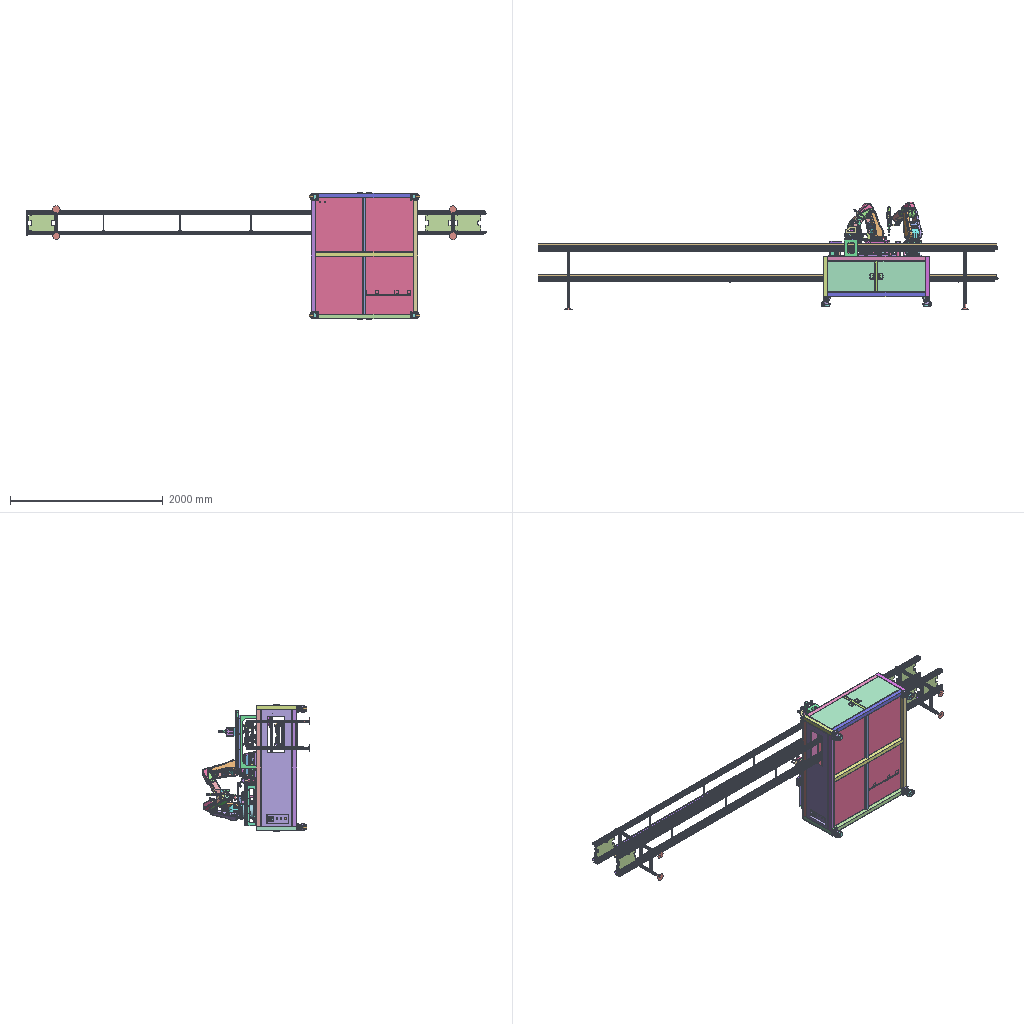Assembly | STEP file | 266 different items | 520 placed | box 6033 x 1412 x 1658 mm
Parts list (item | name | quantity | parent item | size | volume):
1 | ASND-0110-IRB120_3-58_IRC5_Link2_rev0 | x2 | in ASND-0110-B, ASND-0110-B-1 | 144.86 x 219.43 x 390.86 mm | 3910323 mm3
2 | ASND-0110-IRB120_3-58_IRC5_Link5_rev0 | x2 | in ASND-0110-C, ASND-0110-C-1 | 51 x 61.424 x 80.382 mm | 189880 mm3
3 | ASND-0110-IRB120_3-58_IRC5_Link5_rev0-1 | x2 | in ASND-0110-C, ASND-0110-C-1 | 21.5 x 70 x 70 mm | 66105 mm3
4 | ASND-0110-IRB120_3-58_IRC5_Link5_rev0-2 | x2 | in ASND-0110-C, ASND-0110-C-1 | 62.5 x 72 x 82 mm | 291195 mm3
5 | ASND-0110-IRB120_3-58_IRC5_Link4_rev0 | x2 | in ASND-0110-A, ASND-0110-A-1 | 193.368 x 85.5 x 92.955 mm | 549837 mm3
6 | ASND-0110-IRB120_3-58_IRC5_Link3_rev0 | x2 | in ASND-0110-A, ASND-0110-A-1 | 10 x 96 x 96 mm | 36166 mm3
7 | ASND-0110-IRB120_3-58_IRC5_Link4_rev0-1 | x2 | in ASND-0110-A, ASND-0110-A-1 | 111.545 x 11.377 x 37.543 mm | 181.054 mm3
8 | ASND-0110-IRB120_3-58_IRC5_Link4_rev0-2 | x2 | in ASND-0110-A, ASND-0110-A-1 | 186.08 x 124 x 105.45 mm | 774376 mm3
9 | ASND-0110-IRB120_3-58_IRC5_Link3_rev0-1 | x2 | in ASND-0110-E, ASND-0110-E-1 | 233.871 x 115.5 x 188.155 mm | 2907846 mm3
10 | ASND-0110-IRB120_3-58_IRC5_Base_rev0 | x2 | in ASND-0110-First axis, ASND-0110-First axisB | 301.2 x 180.524 x 166.334 mm | 6215073 mm3
11 | ASND-0110-IRB120_3-58_IRC5_Link1_rev0-1 | x2 | in ASND-0110-First axis, ASND-0110-First axisB | 215 x 215 x 22 mm | 381566 mm3
12 | ASND-0110-Body 1-1 | x1 | in ASND-0110-D1 | 280 x 240 x 15 mm | 976987 mm3
13 | ASND-0110-Body 1-2 | x1 | in ASND-0110-D | 280 x 220 x 15 mm | 890688 mm3
14 | ASND-0110-Body 1-5 | x4 | in ASND-0110-asd | 5 x 5 x 2.3 mm | 45.16 mm3
15 | ASND-0110-TPIM-023 | x1 | in ASND-0110-asd | 111.9 x 71.3 x 30 mm | 98030 mm3
16 | ASND-0110-IRB120_Link6_rev0 | x2 | in ASND-0110-Robot suction mechanism, ASND-0110-Screw locking mechanism | 13 x 40 x 40 mm | 13678 mm3
17 | ASND-0110-Body 1-3 | x8 | in ASND-0110-Robot suction mechanism, ASND-0110-XXY mechanism | 20 x 20 x 10 mm | 1461 mm3
18 | ASND-0110-TPIM-022 | x1 | in ASND-0110-Robot suction mechanism | 248.345 x 15 x 75.4 mm | 86870 mm3
19 | ASND-0110-TPIM-020 | x1 | in ASND-0110-Robot suction mechanism | 92 x 92 x 18 mm | 89646 mm3
20 | ASND-0110-YD02 | x2 | in ASND-0110-Robot suction mechanism | 66 x 64 x 12.7 mm | 33292 mm3
21 | ASND-0110-TPIM-068 | x1 | in ASND-0110-Robot suction mechanism | 46.8 x 34.8 x 15.8 mm | 14684 mm3
22 | ASND-0110-Solid1 | x1 | in ASND-0110-Robot suction mechanism | 20.8 x 7 x 7 mm | 257.271 mm3
23 | ASND-0110-TPIM-标定01 | x1 | in ASND-0110-Robot suction mechanism | 24 x 14 x 6 mm | 2012 mm3
24 | ASND-0110-Body 1-4 | x1 | in ASND-0110-Robot suction mechanism | 83 x 53 x 7 mm | 13678 mm3
25 | ASND-0110-HI_Motor--01-APAAa5wgTCTF01 | x1 | in ASND-0110-MAMS012G1ATCTF01 | 117.03 x 38.2 x 38.2 mm | 124253 mm3
26 | ASND-0110-HI_Motoplug--01ATCTF01 | x1 | in ASND-0110-MAMS012G1ATCTF01 | 27 x 33.5 x 37.535 mm | 8192 mm3
27 | ASND-0110-HI_Cabel Motoplug--01PTCTF01 | x1 | in ASND-0110-MAMS012G1ATCTF01 | 9 x 52.5 x 9 mm | 1909 mm3
28 | ASND-0110-HI_Motor ConnectorTCTF01 | x1 | in ASND-0110-MAMS012G1ATCTF01 | 23.7 x 14.7 x 9.8 mm | 1306 mm3
29 | ASND-0110-HI_Encoder--01PTCTF01 | x1 | in ASND-0110-MAMS012G1ATCTF01 | 30.365 x 32.633 x 22.9 mm | 5926 mm3
30 | ASND-0110-HI_Cabel  brake--01-P-4TCTF01 | x1 | in ASND-0110-MAMS012G1ATCTF01 | 7.2 x 36.535 x 7.2 mm | 1162 mm3
31 | ASND-0110-HI_2500 p_r ConnectorTCTF01 | x1 | in ASND-0110-MAMS012G1ATCTF01 | 23.7 x 14.7 x 14.5 mm | 2117 mm3
32 | ASND-0110-KK60-500 | x1 | in ASND-0110-KK60-500A1-F0 | 570 x 44.5 x 60 mm | 511648 mm3
33 | ASND-0110-KK60-A1 | x1 | in ASND-0110-KK60-500A1-F0 | 82 x 21 x 51.857 mm | 53460 mm3
34 | ASND-0110-TCTF01-28 | x1 | in ASND-0110-KK module TCTF01(default-_flexible1) | 12 x 50 x 44 mm | 18847 mm3
35 | ASND-0110-KK6010P-600A1-F1CS1-8TCTF01 | x1 | in ASND-0110-KK module TCTF01(default-_flexible1) | 500 x 8 x 5 mm | 9828 mm3
36 | ASND-0110-HGR15_1TCTF01sb | x1 | in ASND-0110-HGR15_1TCTF01 | 15 x 15 x 530 mm | 97544 mm3
37 | ASND-0110-TCTF01-31 | x1 | in ASND-0110-Tooling mechanism | 90 x 51 x 22 mm | 59920 mm3
38 | ASND-0110-Body 1-9 | x1 | in ASND-0110-Tooling mechanism | 160 x 114 x 12 mm | 207606 mm3
39 | ASND-0110-Body 1-10 | x1 | in ASND-0110-Tooling mechanism | 160 x 114 x 25 mm | 365953 mm3
40 | ASND-0110-DH2TC90-28(2) | x1 | in ASND-0110-Tooling mechanism | 15 x 30 x 16.25 mm | 397.632 mm3
41 | ASND-0110-HGH15_2TCTF01sb | x1 | in ASND-0110-Tooling mechanism | 34 x 23.7 x 61.4 mm | 36561 mm3
42 | ASND-0110-KK60-A1gf4 | x1 | in ASND-0110-Tooling mechanism | 82 x 21 x 51.857 mm | 53460 mm3
43 | - | x1 | in ASND-0110-Tooling mechanism | 13 x 52 x 15.011 mm | 2605 mm3
44 | ASND-0110-Body 1-11 | x1 | in ASND-0110-Tooling mechanism | 80 x 22 x 35 mm | 6854 mm3
45 | ASND-0110-TCTF01-29 | x1 | in ASND-0110-Feeding mechanism | 70 x 101.1 x 530 mm | 1817903 mm3
46 | ASND-0110-TCTF01-34 | x1 | in ASND-0110-Feeding mechanism | 530 x 32 x 127.1 mm | 1195079 mm3
47 | ASND-0110-TCTF01-30(default) | x1 | in ASND-0110-Feeding mechanism | 522 x 1.5 x 56 mm | 43747 mm3
48 | ASND-0110-Body 1-6 | x1 | in ASND-0110-Feeding mechanism | 550 x 32 x 10 mm | 26590 mm3
49 | ASND-0110-Positioning edgeHSG side gTCTF01 | x2 | in ASND-0110-Feeding mechanism | 6 x 6 x 14 mm | 362.314 mm3
50 | ASND-0110-Body 1-7 | x1 | in ASND-0110-Feeding mechanism | 22 x 79.611 x 439.805 mm | 70298 mm3
51 | ASND-0110-Body 1-8 | x1 | in ASND-0110-Feeding mechanism | 202 x 550 x 12 mm | 1322271 mm3
52 | ASND-0110-1 | x2 | in ASND-0110-Rotary clamping mechanism, ASND-0110-Revolve夹持机构-1 | 29 x 29 x 68 mm | 33970 mm3
53 | ASND-0110-clamp 12 | x2 | in ASND-0110-Rotary clamping mechanism, ASND-0110-Revolve夹持机构-1 | 87 x 17 x 20 mm | 14618 mm3
54 | ASND-0110-Body 1-14 | x2 | in ASND-0110-Rotary clamping mechanism, ASND-0110-Revolve夹持机构-1 | 20 x 12 x 2 mm | 472 mm3
55 | ASND-0110-Surface 1-1 | x1 | in ASND-0110-XXY mechanism | - | -
56 | ASND-0110-TCTF01-24 | x1 | in ASND-0110-XXY mechanism | 366.812 x 377.833 x 20 mm | 1326662 mm3
57 | ASND-0110-TCTF01-23 | x1 | in ASND-0110-XXY mechanism | 366.812 x 377.833 x 16 mm | 1379157 mm3
58 | ASND-0110-TCTF01-35 | x1 | in ASND-0110-XXY mechanism | 317.501 x 248.833 x 21 mm | 1208594 mm3
59 | ASND-0110-TCTF01-58 | x1 | in ASND-0110-XXY mechanism | 256.83 x 10 x 30 mm | 53115 mm3
60 | ASND-0110-TCTF01-57 | x1 | in ASND-0110-XXY mechanism | 78 x 30 x 10 mm | 20925 mm3
61 | ASND-0110-TCTF01-57-1 | x1 | in ASND-0110-XXY mechanism | 92 x 30 x 10 mm | 25160 mm3
62 | ASND-0110-Body 1-12 | x2 | in ASND-0110-XXY mechanism | 66 x 29 x 8 mm | 12885 mm3
63 | ASND-0110-Body 1-13 | x1 | in ASND-0110-XXY mechanism | 366.812 x 370.85 x 30 mm | 2210329 mm3
64 | ASND-0110-Solid1-1 | x1 | in ASND-0110-XXY mechanism | 12.3 x 7 x 7 mm | 177.16 mm3
65 | ASND-0110-PG Flea2 | x6 | in ASND-0110-Camera mechanisma, ASND-0110-Camera mechanisma-1, ASND-0110-Camera mechanisma-2, ASND-0110-Camera mechanisma-3, ASND-0110-Camera section, ASND-0110-相机部分-1 | 29 x 29 x 47.1 mm | 26811 mm3
66 | ASND-0110-Body 1-15 | x4 | in ASND-0110-Camera mechanisma, ASND-0110-Camera mechanisma-1, ASND-0110-Camera mechanisma-2, ASND-0110-Camera mechanisma-3 | 40.5 x 29 x 94 mm | 35874 mm3
67 | ASND-0110-Surface 1-2 | x1 | in ASND-0110-tiaoj | - | -
68 | ASND-0110-OPT-CO40-X-V1.0.5 mounting plate | x4 | in ASND-0110-OPT-CO40-X-V1.0.5, ASND-0110-OPT-CO40-X-V1.0.5_1, ASND-0110-OPT-CO40-X-V1.0.5_2, ASND-0110-OPT-CO40-X-V1.0.5_3 | 32 x 39 x 8 mm | 9600 mm3
69 | ASND-0110-OPT-CO40-X-V1.0.5 side plate | x4 | in ASND-0110-OPT-CO40-X-V1.0.5, ASND-0110-OPT-CO40-X-V1.0.5_1, ASND-0110-OPT-CO40-X-V1.0.5_2, ASND-0110-OPT-CO40-X-V1.0.5_3 | 69 x 39 x 4 mm | 10181 mm3
70 | ASND-0110-OPT-CO40-X-V1.0 rear cover plate | x4 | in ASND-0110-OPT-CO40-X-V1.0.5, ASND-0110-OPT-CO40-X-V1.0.5_1, ASND-0110-OPT-CO40-X-V1.0.5_2, ASND-0110-OPT-CO40-X-V1.0.5_3 | 32 x 35 x 5 mm | 5286 mm3
71 | ASND-0110-OPT-CO40-X-V1.0 upper cover plate | x4 | in ASND-0110-OPT-CO40-X-V1.0.5, ASND-0110-OPT-CO40-X-V1.0.5_1, ASND-0110-OPT-CO40-X-V1.0.5_2, ASND-0110-OPT-CO40-X-V1.0.5_3 | 34 x 29 x 2 mm | 1761 mm3
72 | ASND-0110-OPT-CO40-X-V1.0 lower cover plate | x4 | in ASND-0110-OPT-CO40-X-V1.0.5, ASND-0110-OPT-CO40-X-V1.0.5_1, ASND-0110-OPT-CO40-X-V1.0.5_2, ASND-0110-OPT-CO40-X-V1.0.5_3 | 34 x 25.2 x 2 mm | 1591 mm3
73 | ASND-0110-OPT-CO40-X-V1.0 diffuser plate | x4 | in ASND-0110-OPT-CO40-X-V1.0.5, ASND-0110-OPT-CO40-X-V1.0.5_1, ASND-0110-OPT-CO40-X-V1.0.5_2, ASND-0110-OPT-CO40-X-V1.0.5_3 | 34.8 x 34.2 x 2 mm | 2380 mm3
74 | ASND-0110-Mirrored OPT-CO40-X-V1.0 side plate | x4 | in ASND-0110-OPT-CO40-X-V1.0.5, ASND-0110-OPT-CO40-X-V1.0.5_1, ASND-0110-OPT-CO40-X-V1.0.5_2, ASND-0110-OPT-CO40-X-V1.0.5_3 | 69 x 39 x 4 mm | 10181 mm3
75 | ASND-0110-2-core power cable | x4 | in ASND-0110-OPT-CO40-X-V1.0.5, ASND-0110-OPT-CO40-X-V1.0.5_1, ASND-0110-OPT-CO40-X-V1.0.5_2, ASND-0110-OPT-CO40-X-V1.0.5_3 | 15 x 5 x 19.875 mm | 201.3 mm3
76 | ASND-0110-TPIM-067 | x2 | in ASND-0110-Lower light source mechanism | 55.8 x 8 x 39 mm | 15980 mm3
77 | ASND-0110-TPIM-065 | x1 | in ASND-0110-Lower light source mechanism | 160 x 111.5 x 30 mm | 146139 mm3
78 | ASND-0110-TPIM-066 | x1 | in ASND-0110-Lower light source mechanism | 132.4 x 10 x 159 mm | 81070 mm3
79 | ASND-0110-Body 1-16 | x2 | in ASND-0110-Lower camera mechanism | 120 x 120 x 10 mm | 61912 mm3
80 | ASND-0110-Body 1-17 | x1 | in ASND-0110-Lower camera mechanism | 128 x 216 x 10 mm | 155040 mm3
81 | ASND-0110-Body 1-18 | x2 | in ASND-0110-Lower camera mechanism | 30 x 31 x 10 mm | 8202 mm3
82 | ASND-0110-Body 1-19 | x2 | in ASND-0110-Lower camera mechanism | 30 x 31 x 10 mm | 8202 mm3
83 | ASND-0110-Body 1-20 | x1 | in ASND-0110-Lower camera mechanism | 178 x 128 x 72 mm | 360301 mm3
84 | ASND-0110-Body 1-21 | x2 | in ASND-0110-Lower camera mechanism | 80 x 52 x 18 mm | 53842 mm3
85 | ASND-0110-4216100000 | x1 | in ASND-0110-4216100080_ASM | 30 x 30 x 163.75 mm | 53858 mm3
86 | ASND-0110-4216107200 | x1 | in ASND-0110-4216100080_ASM | 25 x 18 x 16 mm | 3261 mm3
87 | ASND-0110-Surface 1-3 | x1 | in ASND-0110-4216100080_ASM | - | -
88 | ASND-0110-4216107480_SPEC | x1 | in ASND-0110-4216100080_ASM | 15.011 x 14 x 14 mm | 1337 mm3
89 | ASND-0110-Surface 1-4 | x1 | in ASND-0110-4216100080_ASM | - | -
90 | ASND-0110-0219110005 | x2 | in ASND-0110-4216100080_ASM | 4.7 x 4.7 x 20 mm | 105.896 mm3
91 | ASND-0110-Surface 1-5 | x2 | in ASND-0110-4216100080_ASM | - | -
92 | ASND-0110-4216101100 | x1 | in ASND-0110-4224300000_ASM | 25 x 116.5 x 18 mm | 12649 mm3
93 | ASND-0110-4216225600 | x1 | in ASND-0110-4224300000_ASM | 29 x 29 x 58 mm | 3832 mm3
94 | ASND-0110-0162110302 | x2 | in ASND-0110-4224300000_ASM | 3 x 3 x 12 mm | 26.529 mm3
95 | ASND-0110-Surface 1-6 | x2 | in ASND-0110-4224300000_ASM | - | -
96 | ASND-0110-0219110003 | x2 | in ASND-0110-4224300000_ASM | 5.5 x 5.5 x 12 mm | 96.355 mm3
97 | ASND-0110-Surface 1-7 | x2 | in ASND-0110-4224300000_ASM | - | -
98 | ASND-0110-0219110001 | x2 | in ASND-0110-4224300000_ASM | 5 x 4.7 x 4.7 mm | 32.246 mm3
99 | ASND-0110-0219110027 | x1 | in ASND-0110-4224300000_ASM | 6 x 6 x 6 mm | 55.363 mm3
100 | ASND-0110-Surface 1-8 | x1 | in ASND-0110-4224300000_ASM | - | -
101 | ASND-0110-4216235500_SPEC | x1 | in ASND-0110-4224300000_ASM | 29.395 x 14.422 x 30 mm | 229.451 mm3
102 | ASND-0110-4216111600 | x1 | in ASND-0110-4224300001_ASM | 9 x 9 x 56.7 mm | 1924 mm3
103 | ASND-0110-4216111500 | x1 | in ASND-0110-4224300001_ASM | 10 x 10 x 6 mm | 119.565 mm3
104 | ASND-0110-4216111700 | x1 | in ASND-0110-4224300001_ASM | 9 x 9 x 9 mm | 120.166 mm3
105 | ASND-0110-0502110051 | x1 | in ASND-0110-4224300001_ASM | 4 x 15.6 x 15.6 mm | 444.035 mm3
106 | ASND-0110-4216109900 | x1 | in ASND-0110-4224300001_ASM | 25 x 25 x 33.65 mm | 5833 mm3
107 | ASND-0110-Surface 1-9 | x1 | in ASND-0110-4224300001_ASM | - | -
108 | ASND-0110-4216111200_SPEC_AF0 | x1 | in ASND-0110-4224300001_ASM | 8.7 x 8.7 x 5.55 mm | 29.663 mm3
109 | ASND-0110-4216111400_AF0 | x1 | in ASND-0110-4224300001_ASM | 8.635 x 8.7 x 1 mm | 17.813 mm3
110 | ASND-0110-Screw gunpart1 | x1 | in ASND-0110-螺丝枪1 | 6.827 x 116 x 6.827 mm | 2290 mm3
111 | ASND-0110-Surface 1-10 | x1 | in ASND-0110-atlas-A | - | -
112 | ASND-0110-Surface 1_1 | x1 | in ASND-0110-atlas-A | - | -
113 | ASND-0110-Surface 1_2 | x1 | in ASND-0110-atlas-A | - | -
114 | ASND-0110-Body 1-22 | x1 | in ASND-0110-Screw locking mechanism | 48 x 48 x 13 mm | 15905 mm3
115 | ASND-0110-Body 1-23 | x1 | in ASND-0110-Screw locking mechanism | 65 x 40 x 6 mm | 15450 mm3
116 | ASND-0110-BAIF-08 | x1 | in ASND-0110-Screw locking mechanism | 104 x 84 x 15 mm | 94605 mm3
117 | ASND-0110-Body 1-1-1 | x1 | in ASND-0110-Screw locking mechanism | 120 x 34 x 8 mm | 32440 mm3
118 | ASND-0110-PG Flea2-1 | x1 | in ASND-0110-Screw locking mechanism | 32 x 32 x 92.1 mm | 40913 mm3
119 | ASND-0110-Body 1-1ww | x1 | in ASND-0110-Screw locking mechanism | 84 x 119.7 x 12 mm | 119908 mm3
120 | ASND-0110-SDS_3 | x1 | in ASND-0110-SDS_SR | 181.1 x 144.1 x 117 mm | 1395902 mm3
121 | ASND-0110-SDS_3_1 | x1 | in ASND-0110-SDS_SR | 1 x 24.6 x 24 mm | 538.331 mm3
122 | ASND-0110-SDS_1 | x1 | in ASND-0110-SDS_SR | 181 x 139 x 3 mm | 64643 mm3
123 | ASND-0110-SDS_2 | x1 | in ASND-0110-SDS_SR | 181 x 139 x 3 mm | 64643 mm3
124 | ASND-0110-SDS_4 | x1 | in ASND-0110-SDS_SR | 122.6 x 80.2 x 5 mm | 16643 mm3
125 | ASND-0110-0162156729 | x16 | in ASND-0110-SDS_SR | 7.5 x 7.5 x 10 mm | 160.064 mm3
126 | ASND-0110-SDS_5 | x1 | in ASND-0110-SDS_SR | 2 x 38.8 x 73.5 mm | 3386 mm3
127 | ASND-0110-SDS_6 | x1 | in ASND-0110-SDS_SR | 31.924 x 31.924 x 2 mm | 1536 mm3
128 | ASND-0110-SDS_7 | x1 | in ASND-0110-SDS_SR | 57.4 x 48.5 x 8.5 mm | 3034 mm3
129 | ASND-0110-SDS_8 | x1 | in ASND-0110-SDS_SR | 22 x 30.4 x 12 mm | 1042 mm3
130 | ASND-0110-SDS_9 | x1 | in ASND-0110-SDS_SR | 21.7 x 12.9 x 40 mm | 1125 mm3
131 | ASND-0110-0211110400 | x2 | in ASND-0110-SDS_SR | 9 x 5.5 x 5.5 mm | 106.119 mm3
132 | ASND-0110-0211110210 | x2 | in ASND-0110-SDS_SR | 6 x 3.8 x 3.8 mm | 33.139 mm3
133 | ASND-0110-0211110266 | x2 | in ASND-0110-SDS_SR | 4.5 x 4.5 x 8.5 mm | 65.135 mm3
134 | ASND-0110-Surface 1-11 | x2 | in ASND-0110-SDS_SR | - | -
135 | ASND-0110-0160099710 | x2 | in ASND-0110-SDS_SR | 3.2 x 3.2 x 4.4 mm | 13.426 mm3
136 | ASND-0110-Surface 1-12 | x2 | in ASND-0110-SDS_SR | - | -
137 | ASND-0110-Body 1-24 | x1 | in ASND-0110-Screw feeding mechanism | 181 x 123 x 100 mm | 983865 mm3
138 | ASND-0110-OPT-CO60-X-V1.0 front cover plate | x2 | in ASND-0110-OPT-CO60-X-V1.0, ASND-0110-OPT-CO60-X-V1.0-1 | 50 x 57.4 x 8 mm | 21783 mm3
139 | ASND-0110-OPT-CO60-X-V1.0 side plate | x2 | in ASND-0110-OPT-CO60-X-V1.0, ASND-0110-OPT-CO60-X-V1.0-1 | 90 x 57.4 x 4 mm | 19730 mm3
140 | ASND-0110-OPT-CO60-X-V1.0 rear cover plate | x2 | in ASND-0110-OPT-CO60-X-V1.0, ASND-0110-OPT-CO60-X-V1.0-1 | 50 x 53 x 5 mm | 13081 mm3
141 | ASND-0110-OPT-CO60-X-V1.0 upper cover plate | x2 | in ASND-0110-OPT-CO60-X-V1.0, ASND-0110-OPT-CO60-X-V1.0-1 | 31 x 52.3 x 2.2 mm | 3229 mm3
142 | ASND-0110-OPT-CO60-X-V1.0 lower cover plate | x2 | in ASND-0110-OPT-CO60-X-V1.0, ASND-0110-OPT-CO60-X-V1.0-1 | 2.2 x 27 x 52.3 mm | 2996 mm3
143 | ASND-0110-2-core outlet terminal | x2 | in ASND-0110-OPT-CO60-X-V1.0, ASND-0110-OPT-CO60-X-V1.0-1 | 27 x 10 x 28.25 mm | 1155 mm3
144 | ASND-0110-Mirrored OPT-CO60-X-V1.0 side plate | x2 | in ASND-0110-OPT-CO60-X-V1.0, ASND-0110-OPT-CO60-X-V1.0-1 | 90 x 57.4 x 4 mm | 19730 mm3
145 | ASND-0110-Body 1-25 | x2 | in ASND-0110-Camera section, ASND-0110-相机部分-1 | 75 x 87.1 x 55 mm | 96917 mm3
146 | ASND-0110-相机连接件2 | x2 | in ASND-0110-Camera section, ASND-0110-相机部分-1 | 75 x 139 x 10 mm | 83120 mm3
147 | ASND-0110-Camera base block | x2 | in ASND-0110-Camera section, ASND-0110-相机部分-1 | 54 x 50 x 14 mm | 21543 mm3
148 | ASND-0110-TPIM-064 | x2 | in ASND-0110-Camera section, ASND-0110-相机部分-1 | 11.6 x 176 x 58 mm | 99143 mm3
149 | ASND-0110-Lens | x2 | in ASND-0110-Camera section, ASND-0110-相机部分-1 | 46 x 141.1 x 46 mm | 154074 mm3
150 | ASND-0110-1-1 | x2 | in ASND-0110-2-25, ASND-0110-2-25-1 | 30 x 30 x 749.1 mm | 248521 mm3
151 | ASND-0110-1-2 | x2 | in ASND-0110-2-25, ASND-0110-2-25-1 | 30 x 30 x 749.1 mm | 248521 mm3
152 | ASND-0110-1-3 | x2 | in ASND-0110-2-25, ASND-0110-2-25-1 | 30 x 320 x 30 mm | 106163 mm3
153 | ASND-0110-1-4 | x4 | in ASND-0110-2-25, ASND-0110-2-25-1 | 30 x 320 x 30 mm | 106163 mm3
154 | ASND-0110-1.120ww | x4 | in ASND-0110-2-25, ASND-0110-2-25-1 | 96.056 x 88 x 96.056 mm | 106190 mm3
155 | ASND-0110-PWP TOP tu pang 20130814.sldasm-Part-1aq (subassembly) | x7 | in ASND-0110-Tray aq, ASND-0110-Tray aq-1, ASND-0110-Tray aq-2, ASND-0110-Tray aq-3, ASND-0110-Tray aq-4, ASND-0110-Tray aq-5, ASND-0110-Tray aq-6 | 256 x 10 x 12 mm | 28147 mm3
156 | ASND-0110-PWP TOP tu pang 20130814.sldasm-Part-2aq (subassembly) | x7 | in ASND-0110-Tray aq, ASND-0110-Tray aq-1, ASND-0110-Tray aq-2, ASND-0110-Tray aq-3, ASND-0110-Tray aq-4, ASND-0110-Tray aq-5, ASND-0110-Tray aq-6 | 337.093 x 249.456 x 14.1 mm | 1124942 mm3
157 | ASND-0110-PWP TOP tu pang 20130814.sldasm-Part-5aq (subassembly) | x7 | in ASND-0110-Tray aq, ASND-0110-Tray aq-1, ASND-0110-Tray aq-2, ASND-0110-Tray aq-3, ASND-0110-Tray aq-4, ASND-0110-Tray aq-5, ASND-0110-Tray aq-6 | 40.426 x 89.575 x 12 mm | 15056 mm3
158 | ASND-0110-PWP TOP tu pang 20130814.sldasm-Part-6aq (subassembly) | x7 | in ASND-0110-Tray aq, ASND-0110-Tray aq-1, ASND-0110-Tray aq-2, ASND-0110-Tray aq-3, ASND-0110-Tray aq-4, ASND-0110-Tray aq-5, ASND-0110-Tray aq-6 | 40.426 x 89.575 x 12 mm | 15056 mm3
159 | ASND-0110-PWP TOP tu pang 20130814.sldasm-Part-7aq (subassembly) | x7 | in ASND-0110-Tray aq, ASND-0110-Tray aq-1, ASND-0110-Tray aq-2, ASND-0110-Tray aq-3, ASND-0110-Tray aq-4, ASND-0110-Tray aq-5, ASND-0110-Tray aq-6 | 31.546 x 101 x 12 mm | 15497 mm3
160 | ASND-0110-PWP TOP tu pang 20130814.sldasm-Part-8aq (subassembly) | x7 | in ASND-0110-Tray aq, ASND-0110-Tray aq-1, ASND-0110-Tray aq-2, ASND-0110-Tray aq-3, ASND-0110-Tray aq-4, ASND-0110-Tray aq-5, ASND-0110-Tray aq-6 | 305.546 x 101 x 12 mm | 72445 mm3
161 | ASND-0110-Q1 | x2 | in ASND-0110-Upper streamline, ASND-0110-Upper流线-1 | 5993 x 32 x 186 mm | 1783036 mm3
162 | ASND-0110-Q2 | x2 | in ASND-0110-Upper streamline, ASND-0110-Upper流线-1 | 6033 x 32.8 x 10 mm | 266115 mm3
163 | ASND-0110-Q3 | x2 | in ASND-0110-Upper streamline, ASND-0110-Upper流线-1 | 6033 x 32.8 x 10 mm | 266115 mm3
164 | ASND-0110-Q20 | x2 | in ASND-0110-Upper streamline, ASND-0110-Upper流线-1 | 11.547 x 10 x 18 mm | 731.296 mm3
165 | ASND-0110-Q20_1 | x2 | in ASND-0110-Upper streamline, ASND-0110-Upper流线-1 | 38 x 16 x 227.5 mm | 31386 mm3
166 | ASND-0110-Q20_2 | x2 | in ASND-0110-Upper streamline, ASND-0110-Upper流线-1 | 11.547 x 10 x 18 mm | 731.296 mm3
167 | ASND-0110-Q21 | x2 | in ASND-0110-Upper streamline, ASND-0110-Upper流线-1 | 11.547 x 10 x 18 mm | 731.296 mm3
168 | ASND-0110-Q21_1 | x2 | in ASND-0110-Upper streamline, ASND-0110-Upper流线-1 | 38 x 16 x 227.5 mm | 31386 mm3
169 | ASND-0110-Q21_2 | x2 | in ASND-0110-Upper streamline, ASND-0110-Upper流线-1 | 11.547 x 10 x 18 mm | 731.296 mm3
170 | ASND-0110-Q22 | x6 | in ASND-0110-Upper streamline, ASND-0110-Upper流线-1 | 11.547 x 10 x 18 mm | 731.296 mm3
171 | ASND-0110-Q22_1 | x6 | in ASND-0110-Upper streamline, ASND-0110-Upper流线-1 | 38 x 16 x 227.5 mm | 31386 mm3
172 | ASND-0110-Q22_2 | x6 | in ASND-0110-Upper streamline, ASND-0110-Upper流线-1 | 11.547 x 10 x 18 mm | 731.296 mm3
173 | ASND-0110-Q23 | x2 | in ASND-0110-Upper streamline, ASND-0110-Upper流线-1 | 40 x 52 x 28.5 mm | 23081 mm3
174 | ASND-0110-Q26 | x2 | in ASND-0110-Upper streamline, ASND-0110-Upper流线-1 | 40 x 52 x 28.5 mm | 23081 mm3
175 | ASND-0110-Q27 | x2 | in ASND-0110-Upper streamline, ASND-0110-Upper流线-1 | 40 x 52 x 28.5 mm | 23081 mm3
176 | ASND-0110-Q29 | x2 | in ASND-0110-Upper streamline, ASND-0110-Upper流线-1 | 6.351 x 5.5 x 2.4 mm | 50.688 mm3
177 | ASND-0110-Q30 | x2 | in ASND-0110-Upper streamline, ASND-0110-Upper流线-1 | 11.5 x 10 x 5 mm | 332.096 mm3
178 | ASND-0110-Q31 | x2 | in ASND-0110-Upper streamline, ASND-0110-Upper流线-1 | 11.5 x 10 x 5 mm | 332.096 mm3
179 | ASND-0110-Q32 | x2 | in ASND-0110-Upper streamline, ASND-0110-Upper流线-1 | 6.351 x 5.5 x 2.4 mm | 50.688 mm3
180 | ASND-0110-Q33 | x2 | in ASND-0110-Upper streamline, ASND-0110-Upper流线-1 | 6.351 x 5.5 x 2.4 mm | 50.688 mm3
181 | ASND-0110-Q34 | x2 | in ASND-0110-Upper streamline, ASND-0110-Upper流线-1 | 11.5 x 10 x 5 mm | 332.096 mm3
182 | ASND-0110-Q35 | x2 | in ASND-0110-Upper streamline, ASND-0110-Upper流线-1 | 11.5 x 10 x 5 mm | 332.096 mm3
183 | ASND-0110-Q36 | x2 | in ASND-0110-Upper streamline, ASND-0110-Upper流线-1 | 6.351 x 5.5 x 2.4 mm | 50.688 mm3
184 | ASND-0110-Q37 | x2 | in ASND-0110-Upper streamline, ASND-0110-Upper流线-1 | 6.351 x 5.5 x 2.4 mm | 50.688 mm3
185 | ASND-0110-Q38 | x2 | in ASND-0110-Upper streamline, ASND-0110-Upper流线-1 | 11.5 x 10 x 5 mm | 332.096 mm3
186 | ASND-0110-Q39 | x2 | in ASND-0110-Upper streamline, ASND-0110-Upper流线-1 | 11.5 x 10 x 5 mm | 332.096 mm3
187 | ASND-0110-Q40 | x2 | in ASND-0110-Upper streamline, ASND-0110-Upper流线-1 | 6.351 x 5.5 x 2.4 mm | 50.688 mm3
188 | ASND-0110-Q1-01 | x2 | in ASND-0110-Upper streamline, ASND-0110-Upper流线-1 | 76 x 32 x 32.35 mm | 32550 mm3
189 | ASND-0110-Q1-01-1 | x2 | in ASND-0110-Upper streamline, ASND-0110-Upper流线-1 | 76 x 32 x 32.35 mm | 32550 mm3
190 | ASND-0110-Q1-01-2 | x2 | in ASND-0110-Upper streamline, ASND-0110-Upper流线-1 | 7.937 x 0.5 x 271.8 mm | 14.332 mm3
191 | ASND-0110-5.1 | x2 | in ASND-0110-Upper streamline, ASND-0110-Upper流线-1 | 44.772 x 36.1 x 6010 mm | 4157112 mm3
192 | ASND-0110-5.2 | x2 | in ASND-0110-Upper streamline, ASND-0110-Upper流线-1 | 44.772 x 36.1 x 6010 mm | 4283109 mm3
193 | ASND-0110-5.3 | x2 | in ASND-0110-Upper streamline, ASND-0110-Upper流线-1 | 30 x 60 x 2960 mm | 1832214 mm3
194 | ASND-0110-5.4 | x4 | in ASND-0110-Upper streamline, ASND-0110-Upper流线-1 | 30 x 60 x 5990 mm | 3707757 mm3
195 | ASND-0110-Q1-1 | x2 | in ASND-0110-Upper streamline, ASND-0110-Upper流线-1 | 7.937 x 0.5 x 1.8 mm | 4.777 mm3
196 | ASND-0110-Q1_1 | x2 | in ASND-0110-Upper streamline, ASND-0110-Upper流线-1 | 5993 x 32 x 129.35 mm | 1768651 mm3
197 | ASND-0110-Q1_2 | x2 | in ASND-0110-Upper streamline, ASND-0110-Upper流线-1 | 7.937 x 0.5 x 1.8 mm | 4.777 mm3
198 | ASND-0110-ACQDS-40x25-G-21aq | x1 | in ASND-0110-ACQDS-40x25-G-2 (200)aq | 75 x 53 x 57 mm | 115109 mm3
199 | ASND-0110-ACQDS-40x25-G-22aq | x1 | in ASND-0110-ACQDS-40x25-G-2 (200)aq | 114 x 40 x 40 mm | 43729 mm3
200 | ASND-0110-ACQDS-40x25-G-23aq | x1 | in ASND-0110-ACQDS-40x25-G-2 (200)aq | 30.5 x 5.725 x 6.069 mm | 552.742 mm3
201 | ASND-0110-ACQDS-40x25-G-24aq | x1 | in ASND-0110-ACQDS-40x25-G-2 (200)aq | 30.5 x 5.725 x 6.069 mm | 552.742 mm3
202 | ASND-0110-6.3aq | x2 | in ASND-0110-a-1aq | 11 x 40 x 18 mm | 7657 mm3
203 | ASND-0110-6.2aq | x1 | in ASND-0110-a-1aq | 357.093 x 212.456 x 12 mm | 877711 mm3
204 | ASND-0110-6.1aq | x4 | in ASND-0110-a-1aq | 60 x 27.1 x 60 mm | 30806 mm3
205 | ASND-0110-6.4aq | x1 | in ASND-0110-a-1aq | 16 x 16 x 200 mm | 40212 mm3
206 | ASND-0110-6.4aq-1 | x1 | in ASND-0110-a-1aq | 16 x 16 x 200 mm | 40212 mm3
207 | ASND-0110-6.4aq-2 | x1 | in ASND-0110-a-1aq | 16 x 16 x 200 mm | 40212 mm3
208 | ASND-0110-6.4aq-3 | x1 | in ASND-0110-a-1aq | 16 x 16 x 200 mm | 40212 mm3
209 | ASND-0110-7.2aq | x1 | in ASND-0110-22-5aq | 20 x 8 x 5 mm | 724.735 mm3
210 | ASND-0110-7.1aq | x1 | in ASND-0110-22-5aq | 6 x 6.928 x 41 mm | 521.465 mm3
211 | ASND-0110-CDQ2B12-5D(0)aq | x1 | in ASND-0110-22-02aq | 25.087 x 25.087 x 56.5 mm | 17303 mm3
212 | ASND-0110-6.5aq | x4 | in ASND-0110-22-02aq | 56 x 41 x 50 mm | 30537 mm3
213 | ASND-0110-Body 1-26 | x1 | in ASND-0110-22-02aq | 10 x 10 x 12 mm | 888.024 mm3
214 | ASND-0110-HGR15_1_1 | x1 | in ASND-0110-HGH_15_ASM_3_ASM | 15 x 15 x 690 mm | 128296 mm3
215 | ASND-0110-KK60-600 | x1 | in ASND-0110-KK60-600A1-F0 | 670 x 44.5 x 60 mm | 591746 mm3
216 | ASND-0110-HI_Motor--01-APAAa5wg | x2 | in ASND-0110-MAMS012G1A, ASND-0110-MAMS012G1A-1 | 117.03 x 38.2 x 38.2 mm | 124253 mm3
217 | ASND-0110-HI_Motoplug--01A | x2 | in ASND-0110-MAMS012G1A, ASND-0110-MAMS012G1A-1 | 27 x 33.5 x 37.535 mm | 8192 mm3
218 | ASND-0110-HI_Cabel Motoplug--01P | x2 | in ASND-0110-MAMS012G1A, ASND-0110-MAMS012G1A-1 | 9 x 52.5 x 9 mm | 1909 mm3
219 | ASND-0110-HI_Motor Connector-3 | x2 | in ASND-0110-MAMS012G1A, ASND-0110-MAMS012G1A-1 | 23.7 x 14.7 x 9.8 mm | 1306 mm3
220 | ASND-0110-HI_Encoder--01P | x2 | in ASND-0110-MAMS012G1A, ASND-0110-MAMS012G1A-1 | 30.365 x 32.633 x 22.9 mm | 5926 mm3
221 | ASND-0110-HI_Cabel  brake--01-P-4 | x2 | in ASND-0110-MAMS012G1A, ASND-0110-MAMS012G1A-1 | 7.2 x 36.535 x 7.2 mm | 1162 mm3
222 | ASND-0110-HI_2500 p_r Connector-3 | x2 | in ASND-0110-MAMS012G1A, ASND-0110-MAMS012G1A-1 | 23.7 x 14.7 x 14.5 mm | 2117 mm3
223 | ASND-0110-KK60-A1-1 | x1 | in ASND-0110-Clamping | 82 x 21 x 51.857 mm | 53460 mm3
224 | ASND-0110-LPMF01-034 | x2 | in ASND-0110-Clamping, ASND-0110-asdwer | 86 x 70 x 19 mm | 72514 mm3
225 | ASND-0110-1-5 | x1 | in ASND-0110-Clamping | 235 x 65 x 70 mm | 504117 mm3
226 | ASND-0110-Body 1-27 | x1 | in ASND-0110-Clamping | 100 x 100 x 282 mm | 364566 mm3
227 | ASND-0110-Body 1-28 | x2 | in ASND-0110-Clamping | 110 x 84 x 12 mm | 78444 mm3
228 | ASND-0110-Body 1-29 | x2 | in ASND-0110-Clamping | 40 x 46 x 32 mm | 43680 mm3
229 | ASND-0110-Body 1-30 | x2 | in ASND-0110-Clamping | 15 x 22 x 40 mm | 9580 mm3
230 | ASND-0110-KK60-150 | x1 | in ASND-0110-KK60-150A1-F0 | 220 x 44.5 x 60 mm | 230513 mm3
231 | ASND-0110-TCTF01-30(default)-2 | x1 | in ASND-0110-KK60-150A1-F0 | 172 x 1.5 x 56 mm | 14347 mm3
232 | ASND-0110-KK60-A1-2 | x1 | in ASND-0110-asdwer | 82 x 21 x 51.857 mm | 53460 mm3
233 | ASND-0110-HGH15_2 | x1 | in ASND-0110-qwresfd | 34 x 23.7 x 61.4 mm | 36561 mm3
234 | ASND-0110-Rubbing imprint | x1 | in ASND-0110-qwresfd | 111 x 175.7 x 16 mm | 311467 mm3
235 | ASND-0110-Part 14989898 | x2 | in ASND-0110-qwresfd | 137.7 x 95 x 15 mm | 127568 mm3
236 | ASND-0110-Part 13g1kk | x1 | in ASND-0110-qwresfd | 111 x 18 x 95 mm | 189810 mm3
237 | ASND-0110-Forehead children guitar | x1 | in ASND-0110-Motor module | 700 x 170 x 215 mm | 5769786 mm3
238 | ASND-0110-偏心销1 | x3 | in ASND-0110-Motor module | 12.8 x 12.8 x 14 mm | 1139 mm3
239 | ASND-0110-LPMF01-028 | x1 | in ASND-0110-Motor module | 170 x 700 x 16 mm | 1565966 mm3
240 | ASND-0110-LPMF01-029 | x1 | in ASND-0110-Motor module | 32 x 700 x 28 mm | 574671 mm3
241 | ASND-0110-TCTF01-30(default)-1 | x1 | in ASND-0110-Motor module | 622 x 1.5 x 56 mm | 52147 mm3
242 | ASND-0110-E63-HLTP01Clogo.sldasm-Part-213 (subassembly) | x4 | in ASND-0110-E63-HLTP01 foot GD-100F(incl. adapter plate), ASND-0110-E63-HLTP01 foot GD-100F(incl. adapter plate)_1, ASND-0110-E63-HLTP01 foot GD-100F(incl. adapter plate)_2, ASND-0110-E63-HLTP01 foot GD-100F(incl. adapter plate)_3 | 70 x 65.311 x 69.5 mm | 134446 mm3
243 | ASND-0110-E63-HLTP01Clogo.sldasm-Part-214 (subassembly) | x4 | in ASND-0110-E63-HLTP01 foot GD-100F(incl. adapter plate), ASND-0110-E63-HLTP01 foot GD-100F(incl. adapter plate)_1, ASND-0110-E63-HLTP01 foot GD-100F(incl. adapter plate)_2, ASND-0110-E63-HLTP01 foot GD-100F(incl. adapter plate)_3 | 30 x 60 x 60 mm | 82218 mm3
244 | ASND-0110-E63-HLTP01Clogo.sldasm-Part-215 (subassembly) | x4 | in ASND-0110-E63-HLTP01 foot GD-100F(incl. adapter plate), ASND-0110-E63-HLTP01 foot GD-100F(incl. adapter plate)_1, ASND-0110-E63-HLTP01 foot GD-100F(incl. adapter plate)_2, ASND-0110-E63-HLTP01 foot GD-100F(incl. adapter plate)_3 | 95 x 101.227 x 100 mm | 310497 mm3
245 | ASND-0110-E63-HLTP01-005 | x4 | in ASND-0110-E63-HLTP01 foot GD-100F(incl. adapter plate), ASND-0110-E63-HLTP01 foot GD-100F(incl. adapter plate)_1, ASND-0110-E63-HLTP01 foot GD-100F(incl. adapter plate)_2, ASND-0110-E63-HLTP01 foot GD-100F(incl. adapter plate)_3 | 95 x 95 x 15 mm | 131850 mm3
246 | ASND-0110-E63-HLTP01标准Lower机架-09 | x4 | in ASND-0110-E63-HLTP0107-02, ASND-0110-E63-HLTP0107-02_1 | 50 x 1580 x 95 mm | 709366 mm3
247 | ASND-0110-E63-HLTP01标准Lower机架-11 | x4 | in ASND-0110-E63-HLTP0107-02, ASND-0110-E63-HLTP0107-02_1 | 50 x 25 x 210 mm | 86940 mm3
248 | ASND-0110-E63-HLTP01 square steel frame | x1 | in ASND-0110-E63-HLTP01 gas spring lower frame | 1400 x 1650 x 525 mm | 1881600 mm3
249 | ASND-0110-E63-HLTP01标准Lower机架-02 | x1 | in ASND-0110-E63-HLTP01 gas spring lower frame | 525 x 1650 x 1280 mm | 4586578 mm3
250 | ASND-0110-E63-HLTP01标准Lower机架-03 | x1 | in ASND-0110-E63-HLTP01 gas spring lower frame | 1400 x 525 x 1530 mm | 5482578 mm3
251 | ASND-0110-E63-HLTP01标准Lower机架-04 | x1 | in ASND-0110-E63-HLTP01 gas spring lower frame | 40 x 40 x 1530 mm | 881280 mm3
252 | ASND-0110-E63-HLTP01标准Lower机架-05 | x1 | in ASND-0110-E63-HLTP01 gas spring lower frame | 40 x 1650 x 405 mm | 466560 mm3
253 | ASND-0110-E63-HLTP01标准Lower机架-06(Default) | x1 | in ASND-0110-E63-HLTP01 gas spring lower frame | 405 x 81.5 x 620 mm | 552144 mm3
254 | ASND-0110-E63-HLTP01标准Lower机架-08 | x1 | in ASND-0110-E63-HLTP01 gas spring lower frame | 26.5 x 408 x 1530 mm | 863375 mm3
255 | ASND-0110-E63-HLTP01-003 | x1 | in ASND-0110-E63-HLTP01 gas spring lower frame | 38 x 405 x 1530 mm | 1141633 mm3
256 | ASND-0110-E63-HLTP01-006 | x1 | in ASND-0110-E63-HLTP01 gas spring lower frame | 257 x 20 x 630 mm | 345415 mm3
257 | ASND-0110-E63-HLTP01标准Lower机架-10 | x1 | in ASND-0110-E63-HLTP01 gas spring lower frame | 1280 x 1530 x 2 mm | 3915543 mm3
258 | ASND-0110-E63-HLTP01power supply C863_PI1#E5830 | x1 | in ASND-0110-E63-HLTP01 gas spring lower frame | 66 x 66 x 39 mm | 89976 mm3
259 | ASND-0110-E63-HLTP01气SpringLower机架.3 | x1 | in ASND-0110-E63-HLTP01 gas spring lower frame | 60 x 60 x 1280 mm | 1146880 mm3
260 | ASND-0110-E63-HLTP01JSC-700 SA | x4 | in ASND-0110-E63-HLTP01 gas spring lower frame | 200 x 200 x 125 mm | 2019631 mm3
261 | ASND-0110-E63-HLTP01气SpringLower机架.4 | x3 | in ASND-0110-E63-HLTP01 gas spring lower frame | 405 x 25 x 620 mm | 418564 mm3
262 | ASND-0110-E63-HLTP01 control board connecting block | x6 | in ASND-0110-E63-HLTP01 gas spring lower frame | 42 x 42 x 50 mm | 8638 mm3
263 | ASND-0110-E63-HLTP01Grip handle UWAUNJ80 | x4 | in ASND-0110-E63-HLTP01 gas spring lower frame | 80 x 30 x 60 mm | 51881 mm3
264 | ASND-0110-Body 1 | x1 | in ASND-0110-00 | 1280 x 1530 x 30 mm | 56875320 mm3
265 | ASND-0110-IRB120_3-58_IRC5_Link1_rev0 | x2 | in ASND-0110-00 | 215 x 217 x 176 mm | 2685979 mm3
266 | ASND-0110-TPIM-069 | x1 | in ASND-0110-00 | 18 x 50 x 80 mm | 7556 mm3
Placements (level | parent | child | x y z in mm | rotation matrix by rows), first 124 of 600 lines:
1 | ASND-0110-00 | ASND-0110-B | -312.504 175.694 -203.563 | -0.277 0.8033 0.5272 0.5061 -0.3444 0.7907 0.8168 0.4858 -0.3112
2 | ASND-0110-B | ASND-0110-IRB120_3-58_IRC5_Link2_rev0 | -202.729 137.976 135.198 | 0.4413 0.5626 0.6991 -0.3003 0.8267 -0.4758 -0.8456 0 0.5338
1 | ASND-0110-00 | ASND-0110-C | -845.184 288.442 110.809 | 0.426 -0.9047 0 0 0 1 -0.9047 -0.426 0
2 | ASND-0110-C | ASND-0110-IRB120_3-58_IRC5_Link5_rev0 | -157.149 106.955 509.558 | 0 0.5626 0.8267 0 0.8267 -0.5626 -1 0 -0
2 | ASND-0110-C | ASND-0110-IRB120_3-58_IRC5_Link5_rev0-1 | 988.855 -169.765 509.558 | 0 0.1234 -0.9924 0 -0.9924 -0.1234 -1 0 0
2 | ASND-0110-C | ASND-0110-IRB120_3-58_IRC5_Link5_rev0-2 | -157.149 106.955 509.558 | 0 0.5626 0.8267 0 0.8267 -0.5626 -1 0 -0
1 | ASND-0110-00 | ASND-0110-A | -735.491 868.72 46.071 | -0.105 -0.5433 0.8329 -0.7996 0.5442 0.2541 -0.5913 -0.6393 -0.4916
2 | ASND-0110-A | ASND-0110-IRB120_3-58_IRC5_Link4_rev0 | -212.21 144.429 154.19 | 0.4133 0.5626 0.716 -0.2813 0.8267 -0.4873 -0.8661 0 0.4999
2 | ASND-0110-A | ASND-0110-IRB120_3-58_IRC5_Link3_rev0 | -212.21 144.429 154.19 | 0.4133 0.5626 0.716 -0.2813 0.8267 -0.4873 -0.8661 0 0.4999
2 | ASND-0110-A | ASND-0110-IRB120_3-58_IRC5_Link4_rev0-1 | -134.481 240.042 160.228 | 0.4133 0.6914 0.5926 -0.2813 0.7159 -0.6391 -0.8661 0.09742 0.4903
2 | ASND-0110-A | ASND-0110-IRB120_3-58_IRC5_Link4_rev0-2 | -212.21 144.429 154.19 | 0.4133 0.5626 0.716 -0.2813 0.8267 -0.4873 -0.8661 0 0.4999
1 | ASND-0110-00 | ASND-0110-E | -148.048 179.761 -300.621 | -0.4008 0.8876 0.2272 0.2181 -0.1484 0.9646 0.8899 0.4361 -0.1341
2 | ASND-0110-E | ASND-0110-IRB120_3-58_IRC5_Link3_rev0-1 | -212.21 144.429 154.19 | 0.4133 0.5626 0.716 -0.2813 0.8267 -0.4873 -0.8661 0 0.4999
1 | ASND-0110-00 | ASND-0110-D1 | -159.61 115.0 -293.797 | 1 0 0 0 0 1 0 -1 0
2 | ASND-0110-D1 | ASND-0110-First axis | -0.0 0.0 -0.0 | -1 0 0 0 -1 0 0 0 1
3 | ASND-0110-First axis | ASND-0110-IRB120_3-58_IRC5_Base_rev0 | -0.0 -0.0 -0.0 | 1 0 0 0 1 0 0 0 1
3 | ASND-0110-First axis | ASND-0110-IRB120_3-58_IRC5_Link1_rev0-1 | -0.0 -0.0 -0.0 | 0.8267 0.5626 0 -0.5626 0.8267 0 0 0 1
2 | ASND-0110-D1 | ASND-0110-Body 1-1 | -140.0 110.0 -3.0 | 1 0 0 0 -1 0 0 0 -1
1 | ASND-0110-00 | ASND-0110-B-1 | 225.1 191.152 105.689 | -0.8015 -0.4763 0.3615 0.5584 -0.38 0.7374 -0.2138 0.7929 0.5706
2 | ASND-0110-B-1 | ASND-0110-IRB120_3-58_IRC5_Link2_rev0 | -202.729 137.976 135.198 | 0.4413 0.5626 0.6991 -0.3003 0.8267 -0.4758 -0.8456 0 0.5338
1 | ASND-0110-00 | ASND-0110-C-1 | -106.038 395.679 -416.97 | 0.9177 0.3972 0 0 0 1 0.3972 -0.9177 0
2 | ASND-0110-C-1 | ASND-0110-IRB120_3-58_IRC5_Link5_rev0 | -157.149 106.955 509.558 | 0 0.5626 0.8267 0 0.8267 -0.5626 -1 0 -0
2 | ASND-0110-C-1 | ASND-0110-IRB120_3-58_IRC5_Link5_rev0-1 | 988.855 -169.765 509.558 | 0 0.1234 -0.9924 0 -0.9924 -0.1234 -1 0 0
2 | ASND-0110-C-1 | ASND-0110-IRB120_3-58_IRC5_Link5_rev0-2 | -157.149 106.955 509.558 | 0 0.5626 0.8267 0 0.8267 -0.5626 -1 0 -0
1 | ASND-0110-00 | ASND-0110-A-1 | 40.779 1060.601 -185.238 | 0.434 0.7265 0.5329 -0.8231 0.5602 -0.09336 -0.3663 -0.3981 0.841
2 | ASND-0110-A-1 | ASND-0110-IRB120_3-58_IRC5_Link4_rev0 | -212.21 144.429 154.19 | 0.4133 0.5626 0.716 -0.2813 0.8267 -0.4873 -0.8661 0 0.4999
2 | ASND-0110-A-1 | ASND-0110-IRB120_3-58_IRC5_Link3_rev0 | -212.21 144.429 154.19 | 0.4133 0.5626 0.716 -0.2813 0.8267 -0.4873 -0.8661 0 0.4999
2 | ASND-0110-A-1 | ASND-0110-IRB120_3-58_IRC5_Link4_rev0-1 | -134.481 240.042 160.228 | 0.4133 0.6914 0.5926 -0.2813 0.7159 -0.6391 -0.8661 0.09742 0.4903
2 | ASND-0110-A-1 | ASND-0110-IRB120_3-58_IRC5_Link4_rev0-2 | -212.21 144.429 154.19 | 0.4133 0.5626 0.716 -0.2813 0.8267 -0.4873 -0.8661 0 0.4999
1 | ASND-0110-00 | ASND-0110-E-1 | 257.067 179.336 156.145 | -0.8361 -0.4528 0.3098 0.4786 -0.3257 0.8154 -0.2683 0.83 0.489
2 | ASND-0110-E-1 | ASND-0110-IRB120_3-58_IRC5_Link3_rev0-1 | -212.21 144.429 154.19 | 0.4133 0.5626 0.716 -0.2813 0.8267 -0.4873 -0.8661 0 0.4999
1 | ASND-0110-00 | ASND-0110-D | 329.934 115.0 271.155 | 0 -1 0 0 0 1 -1 0 -0
2 | ASND-0110-D | ASND-0110-First axisB | -0.0 -0.0 -0.0 | 1 0 0 0 1 0 0 0 1
3 | ASND-0110-First axisB | ASND-0110-IRB120_3-58_IRC5_Base_rev0 | -0.0 -0.0 -0.0 | 1 0 0 0 1 0 0 0 1
3 | ASND-0110-First axisB | ASND-0110-IRB120_3-58_IRC5_Link1_rev0-1 | -0.0 -0.0 -0.0 | 0.8267 0.5626 0 -0.5626 0.8267 0 0 0 1
2 | ASND-0110-D | ASND-0110-Body 1-2 | -140.0 110.0 -3.0 | 1 0 0 0 -1 0 0 0 -1
1 | ASND-0110-00 | ASND-0110-Robot suction mechanism | -477.346 328.93 86.616 | 0.9997 -0.02599 0 0 0 1 -0.02599 -0.9997 0
2 | ASND-0110-Robot suction mechanism | ASND-0110-asd | -0.0 -0.0 -0.0 | 1 0 0 0 1 0 0 0 1
3 | ASND-0110-asd | ASND-0110-Body 1-5 | -38.02 -0.714 -18.93 | 1 -0.000237 0 -0.000237 -1 0 0 0 -1
3 | ASND-0110-asd | ASND-0110-Body 1-5 | 59.947 -3.26 -18.93 | 1 -0.000235 0 -0.000235 -1 0 0 0 -1
3 | ASND-0110-asd | ASND-0110-Body 1-5 | -36.798 46.27 -18.93 | 1 -0.008905 0 -0.008905 -1 0 0 0 -1
3 | ASND-0110-asd | ASND-0110-Body 1-5 | 61.168 43.724 -18.93 | 1 0.003823 0 0.003823 -1 0 0 0 -1
3 | ASND-0110-asd | ASND-0110-TPIM-023 | 7.245 -1.14 -20.93 | -0.9997 0.02599 0 0.02599 0.9997 0 0 0 -1
2 | ASND-0110-Robot suction mechanism | ASND-0110-IRB120_Link6_rev0 | -613.598 215.41 469.07 | 0 0.02599 0.9997 0 0.9997 -0.02599 -1 0 -0
2 | ASND-0110-Robot suction mechanism | ASND-0110-Body 1-3 | -6.095 15.212 -12.23 | 0.993 0.1184 0 0.1184 -0.993 0 0 0 -1
2 | ASND-0110-Robot suction mechanism | ASND-0110-Body 1-3 | 29.491 37.295 -12.23 | 0.996 -0.08974 0 -0.08974 -0.996 0 0 0 -1
2 | ASND-0110-Robot suction mechanism | ASND-0110-Body 1-3 | -5.497 38.204 -12.23 | 0.9766 -0.2149 0 -0.2149 -0.9766 0 0 0 -1
2 | ASND-0110-Robot suction mechanism | ASND-0110-Body 1-3 | 28.893 14.302 -12.23 | 0.9438 0.3304 0 0.3304 -0.9438 0 0 0 -1
2 | ASND-0110-Robot suction mechanism | ASND-0110-TPIM-022 | 5.054 59.282 -22.93 | 0.02599 0 0.9997 0.9997 0 -0.02599 0 1 0
2 | ASND-0110-Robot suction mechanism | ASND-0110-TPIM-020 | 16.189 199.04 81.07 | -0.9997 -0.02599 0 0.02599 -0.9997 0 0 0 1
2 | ASND-0110-Robot suction mechanism | ASND-0110-YD02 | -8.153 224.681 17.07 | -0.02599 0 -0.9997 -0.9997 0 0.02599 0 1 -0
2 | ASND-0110-Robot suction mechanism | ASND-0110-YD02 | 54.526 223.052 17.07 | -0.02599 0 -0.9997 -0.9997 0 0.02599 0 1 -0
2 | ASND-0110-Robot suction mechanism | ASND-0110-TPIM-068 | 7.245 -1.14 -2.93 | 0.9997 0.02599 0 -0.02599 0.9997 0 0 0 1
2 | ASND-0110-Robot suction mechanism | ASND-0110-Solid1 | -5.497 38.204 -16.23 | 0 -0.2477 0.9688 0 -0.9688 -0.2477 1 0 0
2 | ASND-0110-Robot suction mechanism | ASND-0110-TPIM-标定01 | 9.975 49.301 -32.83 | 0.9997 -0.02599 0 -0.02599 -0.9997 0 0 0 -1
2 | ASND-0110-Robot suction mechanism | ASND-0110-Body 1-4 | -30.399 3.84 -23.93 | 0.9997 0.02599 0 -0.02599 0.9997 0 0 0 1
1 | ASND-0110-00 | ASND-0110-Feeding mechanism | -569.0 110.1 -335.0 | -1 0 0 0 -1 0 0 0 1
2 | ASND-0110-Feeding mechanism | ASND-0110-KK module TCTF01(default-_flexible1) | 151.0 2.909 11.0 | -1 0 0 0 -1 0 0 0 1
3 | ASND-0110-KK module TCTF01(default-_flexible1) | ASND-0110-MAMS012G1ATCTF01 | 0.0 128.909 421.0 | 0 -1 0 0 0 1 -1 0 0
4 | ASND-0110-MAMS012G1ATCTF01 | ASND-0110-HI_Motor--01-APAAa5wgTCTF01 | -6.0 0.0 -0.0 | 1 0 0 0 1 0 0 0 1
4 | ASND-0110-MAMS012G1ATCTF01 | ASND-0110-HI_Motoplug--01ATCTF01 | -40.8 19.0 0.0 | 0 0 -1 0 1 0 1 0 -0
4 | ASND-0110-MAMS012G1ATCTF01 | ASND-0110-HI_Cabel Motoplug--01PTCTF01 | -31.3 32.5 0.0 | 0 0 -1 0 1 0 1 0 -0
4 | ASND-0110-MAMS012G1ATCTF01 | ASND-0110-HI_Motor ConnectorTCTF01 | -31.3 96.9 0.0 | 0 -1 0 -1 0 0 0 0 -1
4 | ASND-0110-MAMS012G1ATCTF01 | ASND-0110-HI_Encoder--01PTCTF01 | -92.0 19.0 0.0 | 1 0 0 0 1 0 0 0 1
4 | ASND-0110-MAMS012G1ATCTF01 | ASND-0110-HI_Cabel  brake--01-P-4TCTF01 | -63.73 31.065 0.0 | 1 0 0 0 1 0 0 0 1
4 | ASND-0110-MAMS012G1ATCTF01 | ASND-0110-HI_2500 p_r ConnectorTCTF01 | -63.73 95.465 0.0 | 0 -1 0 -1 0 0 0 0 -1
3 | ASND-0110-KK module TCTF01(default-_flexible1) | ASND-0110-KK60-500A1-F0 | 0.0 105.909 350.0 | 0 0 -1 0 1 0 1 0 0
4 | ASND-0110-KK60-500A1-F0 | ASND-0110-KK60-500 | -0.0 -0.0 -0.0 | 1 0 0 0 1 0 0 0 1
4 | ASND-0110-KK60-500A1-F0 | ASND-0110-KK60-A1 | -0.0 -0.0 -0.0 | 1 0 0 0 1 0 0 0 1
3 | ASND-0110-KK module TCTF01(default-_flexible1) | ASND-0110-TCTF01-28 | 0.0 128.909 409.0 | 0 1 0 0 0 1 1 0 0
3 | ASND-0110-KK module TCTF01(default-_flexible1) | ASND-0110-KK6010P-600A1-F1CS1-8TCTF01 | 12.85 105.0 150.0 | 0 0 -1 0 -1 0 -1 0 0
2 | ASND-0110-Feeding mechanism | ASND-0110-HGR15_1TCTF01 | 56.5 -142.0 235.0 | -1 0 0 0 -1 0 0 0 1
3 | ASND-0110-HGR15_1TCTF01 | ASND-0110-HGR15_1TCTF01sb | -0.0 -0.0 -0.0 | 1 0 0 0 1 0 0 0 1
2 | ASND-0110-Feeding mechanism | ASND-0110-Tooling mechanism | -0.0 2.909 19.802 | 1 0 0 0 1 0 0 0 1
3 | ASND-0110-Tooling mechanism | ASND-0110-TCTF01-31 | 151.0 -137.909 243.705 | -1 0 0 0 0 -1 0 -1 -0
3 | ASND-0110-Tooling mechanism | ASND-0110-Body 1-9 | 36.0 -157.909 161.205 | 1 0 0 0 0 -1 0 1 -0
3 | ASND-0110-Tooling mechanism | ASND-0110-Body 1-10 | 36.0 -179.909 161.205 | 1 0 0 0 0 -1 0 1 -0
3 | ASND-0110-Tooling mechanism | ASND-0110-DH2TC90-28(2) | 144.5 -140.909 -49.795 | 0 0 1 0 -1 0 1 0 0
3 | ASND-0110-Tooling mechanism | ASND-0110-HGH15_2TCTF01sb | 56.5 -144.909 218.205 | -1 0 0 0 -1 0 0 0 1
3 | ASND-0110-Tooling mechanism | ASND-0110-KK60-A1gf4 | 151.0 -105.909 297.205 | 0 0 1 0 -1 0 1 0 0
3 | ASND-0110-Tooling mechanism | subassembly 2 | 96.0 -189.909 228.205 | 1 0 0 0 1 0 0 0 1
3 | ASND-0110-Tooling mechanism | ASND-0110-Body 1-11 | 89.0 -169.909 278.205 | 0 1 0 1 0 0 0 0 -1
2 | ASND-0110-Feeding mechanism | ASND-0110-TCTF01-29 | 156.0 0.0 -0.0 | -1 0 0 0 -1 0 0 0 1
2 | ASND-0110-Feeding mechanism | ASND-0110-TCTF01-34 | 70.0 -72.0 95.0 | 0 -1 0 0 0 -1 1 0 0
2 | ASND-0110-Feeding mechanism | ASND-0110-TCTF01-30(default) | 151.0 -149.0 12.5 | 0 0 1 0 -1 0 1 0 0
2 | ASND-0110-Feeding mechanism | ASND-0110-Body 1-6 | 115.0 -1.9 -150.0 | 0 -1 0 0 0 -1 1 0 0
2 | ASND-0110-Feeding mechanism | ASND-0110-Positioning edgeHSG side gTCTF01 | 184.0 -99.0 320.0 | 0 -1 0 0 0 -1 1 0 0
2 | ASND-0110-Feeding mechanism | ASND-0110-Positioning edgeHSG side gTCTF01 | 184.0 -99.0 -90.0 | 0.4183 -0.9083 0 0 0 -1 0.9083 0.4183 0
2 | ASND-0110-Feeding mechanism | ASND-0110-Body 1-7 | 111.0 -2.9 -20.0 | -1 0 0 0 -1 0 0 0 1
2 | ASND-0110-Feeding mechanism | ASND-0110-Body 1-8 | 9.0 -1.9 400.0 | 1 0 0 0 0 1 0 -1 -0
1 | ASND-0110-00 | ASND-0110-XXY mechanism | -140.007 86.0 359.874 | 1 0 0 0 -1 0 0 0 -1
2 | ASND-0110-XXY mechanism | ASND-0110-Rotary clamping mechanism | -0.2242 0.0 393.616 | -1 0 0 0 1 0 0 0 -1
3 | ASND-0110-Rotary clamping mechanism | ASND-0110-1 | -50.543 -199.5 202.391 | 1 0 0 0 0 -1 0 1 -0
3 | ASND-0110-Rotary clamping mechanism | ASND-0110-clamp 12 | -50.543 -209.8 202.391 | -1 0 0 0 -1 0 0 0 1
3 | ASND-0110-Rotary clamping mechanism | ASND-0110-Body 1-14 | -107.543 -218.5 196.391 | -1 0 0 0 0 1 0 1 0
2 | ASND-0110-XXY mechanism | ASND-0110-Revolve夹持机构-1 | -0.6384 0.0 -11.167 | 1 0 0 0 1 0 0 0 1
3 | ASND-0110-Revolve夹持机构-1 | ASND-0110-1 | -50.543 -199.5 202.391 | 1 0 0 0 0 -1 0 1 -0
3 | ASND-0110-Revolve夹持机构-1 | ASND-0110-clamp 12 | -50.543 -209.8 202.391 | -1 0 0 0 -1 0 0 0 1
3 | ASND-0110-Revolve夹持机构-1 | ASND-0110-Body 1-14 | -107.543 -218.5 196.391 | -1 0 0 0 0 1 0 1 0
2 | ASND-0110-XXY mechanism | ASND-0110-Body 1-3 | -110.0 -202.3 121.724 | 0.8765 0.4814 0 0 0 -1 -0.4814 0.8765 -0
2 | ASND-0110-XXY mechanism | ASND-0110-Body 1-3 | 110.0 -202.3 121.724 | 0.9622 0.2723 0 0 0 -1 -0.2723 0.9622 -0
2 | ASND-0110-XXY mechanism | ASND-0110-Body 1-3 | -110.0 -202.3 91.724 | 1 0 0 0 0 -1 0 1 -0
2 | ASND-0110-XXY mechanism | ASND-0110-Body 1-3 | 110.0 -202.3 91.724 | 1 0 0 0 0 -1 0 1 -0
2 | ASND-0110-XXY mechanism | ASND-0110-Surface 1-1 | 0.0071 -14.0 114.874 | 1 0 0 0 -1 0 0 0 -1
2 | ASND-0110-XXY mechanism | ASND-0110-TCTF01-24 | -2.681 -170.0 -89.849 | -1 0 0 0 0 -1 0 -1 -0
2 | ASND-0110-XXY mechanism | ASND-0110-TCTF01-23 | -2.501 -154.0 -74.846 | -1 0 0 0 0 -1 0 -1 -0
2 | ASND-0110-XXY mechanism | ASND-0110-TCTF01-35 | -0.0 -190.0 42.549 | -1 0 0 0 0 -1 0 -1 -0
2 | ASND-0110-XXY mechanism | ASND-0110-TCTF01-58 | 166.82 -205.0 20.809 | 0 -1 0 0 0 -1 1 0 -0
2 | ASND-0110-XXY mechanism | ASND-0110-TCTF01-57 | -227.64 -205.0 156.724 | -1 0 0 0 -1 0 0 0 1
2 | ASND-0110-XXY mechanism | ASND-0110-TCTF01-57-1 | 0.0 -205.0 156.724 | -1 0 0 0 -1 0 0 0 1
2 | ASND-0110-XXY mechanism | ASND-0110-Body 1-12 | -96.681 -146.0 176.724 | 1 0 0 0 0 -1 0 1 -0
2 | ASND-0110-XXY mechanism | ASND-0110-Body 1-12 | 95.819 -146.0 205.724 | -1 0 0 0 0 -1 0 -1 -0
2 | ASND-0110-XXY mechanism | ASND-0110-Body 1-13 | -199.993 -124.0 -85.126 | 1 0 0 0 0 -1 0 1 -0
2 | ASND-0110-XXY mechanism | ASND-0110-Solid1-1 | -110.0 -206.3 121.724 | 0 0.004839 1 1 0 0 0 1 -0.004839
1 | ASND-0110-00 | ASND-0110-Lower camera mechanism | -0.0 -0.0 -0.0 | 1 0 0 0 1 0 0 0 1
2 | ASND-0110-Lower camera mechanism | ASND-0110-Camera mechanisma | 154.664 -40.505 574.551 | 0 1 0 1 0 0 0 0 -1
3 | ASND-0110-Camera mechanisma | ASND-0110-PG Flea2 | 139.13 -344.864 362.5 | 0 0 1 1 0 0 0 1 -0
3 | ASND-0110-Camera mechanisma | ASND-0110-Body 1-15 | 272.23 -344.864 362.5 | 0 0 -1 0 1 0 1 0 0
2 | ASND-0110-Lower camera mechanism | ASND-0110-Camera mechanisma-1 | -535.064 -40.505 -78.649 | 0 -1 0 1 0 0 0 0 1
3 | ASND-0110-Camera mechanisma-1 | ASND-0110-PG Flea2 | 139.13 -344.864 362.5 | 0 0 1 1 0 0 0 1 -0
3 | ASND-0110-Camera mechanisma-1 | ASND-0110-Body 1-15 | 272.23 -344.864 362.5 | 0 0 -1 0 1 0 1 0 0
2 | ASND-0110-Lower camera mechanism | ASND-0110-Camera mechanisma-2 | -434.664 -40.505 -78.649 | 0 -1 0 1 0 0 0 0 1
3 | ASND-0110-Camera mechanisma-2 | ASND-0110-PG Flea2 | 139.13 -344.864 362.5 | 0 0 1 1 0 0 0 1 -0
3 | ASND-0110-Camera mechanisma-2 | ASND-0110-Body 1-15 | 272.23 -344.864 362.5 | 0 0 -1 0 1 0 1 0 0